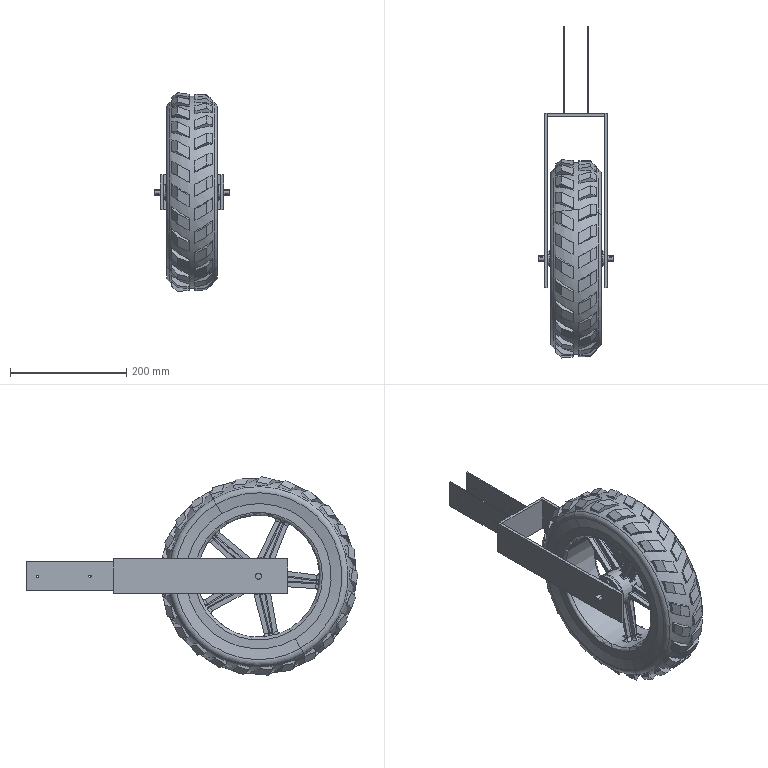Part | SolidWorks | features CompositeCurve 1, MirrorCompFeat 1, ReferencePattern 1 | 11 solids | 1010 faces | box 130 x 571.206 x 341.736 mm | volume 2047297 mm3 | plane 450 | cylinder 202 | sphere 148 | spline 110 | torus 88 | cone 12 | commonest cylinder face diameters 4 x67 10 x49 8 x12 17.4 x8 23.8 x8 30 x8